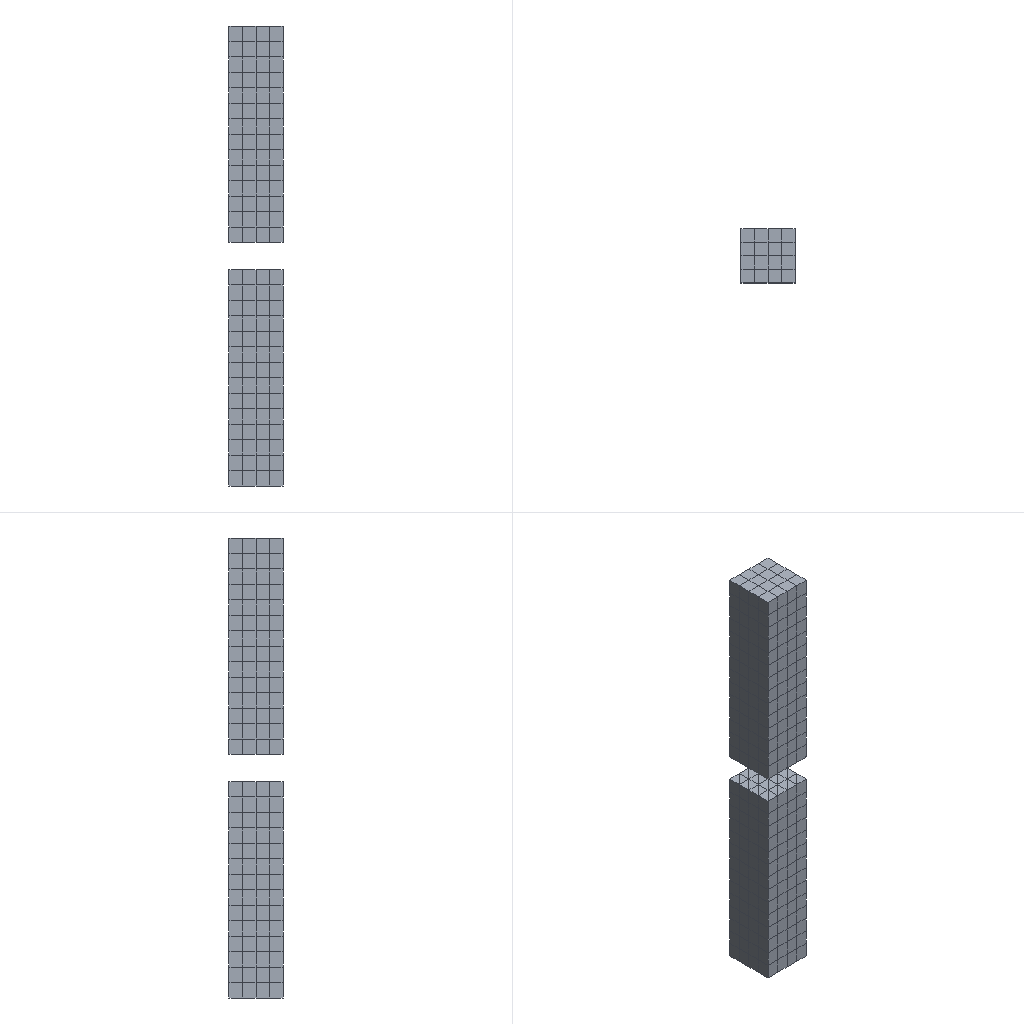Simulation study | ansys workbench
Ansys APDL input file, long lists of numbers shortened:
/batch
/config,noeldb,1     ! force off writing results to database
*get,_wallstrt,active,,time,wall
! ANSYS input file written by Workbench version 16.0 RELEASE
! File used for geometry attach: C:\Users\USE\AppData\Local\Temp\WB_LAPTOP-92PEKBNI_hmm_2756_2\unsaved_project_files\dp0\SYS\DM\SYS.agdb
/title,unsaved_project--Transient (B5)
*DIM,_wb_ProjectScratch_dir,string,248
_wb_ProjectScratch_dir(1) = 'C:\Users\USE\AppData\Local\Temp\WB_LAPTOP-92PEKBNI_hmm_2756_2\_ProjectScratch\Scr97FA\'
*DIM,_wb_SolverFiles_dir,string,248
_wb_SolverFiles_dir(1) = 'C:\Users\USE\AppData\Local\Temp\WB_LAPTOP-92PEKBNI_hmm_2756_2\unsaved_project_files\dp0\SYS-1\MECH\'
*DIM,_wb_userfiles_dir,string,248
_wb_userfiles_dir(1) = 'C:\Users\USE\AppData\Local\Temp\WB_LAPTOP-92PEKBNI_hmm_2756_2\unsaved_project_files\user_files\'
/com,--- Data in consistent NMM units. See Solving Units in the help system for more information.
/units,MPA
/nopr
/wb,file,start              !  signify a WB generated input file
/prep7
! Turn off shape checking because checks already performed inside WB mesher.
! See help system for more information.
SHPP,OFF,,NOWARN
/nolist
etcon,set             ! allow ANSYS to choose best KEYOP's for 180x elements
/com,*********** Nodes for the whole assembly ***********
nblock,3
(1i9,3e20.9e3)
        1   -2.500000000E+000    2.500000000E+000    2.857142857E+000
! (2649 more lines like these left out)
-1
/wb,elem,start            !  set before creation of elements
/com,*********** Elements for Body 1 "Solid" ***********
et,1,186
keyo,1,2,1          ! set full integration on SOLID186
eblock,19,solid,,224
(19i9)
        1        1        1        1        0        0        0        0       20        0        1        1      366      286      270      156      375      287      283
! (447 more lines like these left out)
-1
/com,*********** Elements for Body 2 "Solid" ***********
et,2,186
keyo,2,2,1          ! set full integration on SOLID186
eblock,19,solid,,224
(19i9)
        2        2        2        2        0        0        0        0       20        0      225     1326     1679     1615     1557     1481     1688     1616     1596
! (447 more lines like these left out)
-1
/wb,elem,end               !  done creating elements
/com,*********** Send User Defined Coordinate System(s) ***********
csys,0
toffst,273.15,  ! Temperature offset from absolute zero
/com,*********** Set Reference Temperature ***********
tref,22.
/wb,mat,start              !  starting to send materials
/com,*********** Send Materials ***********
MP,DENS,1,7.85e-09,	! tonne mm^-3
MP,ALPX,1,1.2e-05,	! C^-1
MP,C,1,434000000,	! mm^2 s^-2 C^-1
MP,KXX,1,60.5,	! tonne mm s^-3 C^-1
MP,RSVX,1,0.00017,	! ohm mm
MP,EX,1,200000,	! tonne s^-2 mm^-1
MP,NUXY,1,0.3,
MP,MURX,1,10000,
MP,DENS,2,7.85e-09,	! tonne mm^-3
MP,ALPX,2,1.2e-05,	! C^-1
MP,C,2,434000000,	! mm^2 s^-2 C^-1
MP,KXX,2,60.5,	! tonne mm s^-3 C^-1
MP,RSVX,2,0.00017,	! ohm mm
MP,EX,2,200000,	! tonne s^-2 mm^-1
MP,NUXY,2,0.3,
MP,MURX,2,10000,
/wb,mat,end                !  done sending materials
!************************* Model Summary ********************
!Solid,	Structural Steel,	matid,	1
!Solid,	Structural Steel,	matid,	2
!************************* End Model Summary ********************
! get the diagonal of the bounding box. Needed later for other things
*get,_xmin,node,,mnloc,x
*get,_ymin,node,,mnloc,y
*get,_zmin,node,,mnloc,z
*get,_xmax,node,,mxloc,x
*get,_ymax,node,,mxloc,y
*get,_zmax,node,,mxloc,z
_ASMDIAG=(_xmax-_xmin)*(_xmax-_xmin)+(_ymax-_ymin)*(_ymax-_ymin)+(_zmax-_zmin)*(_zmax-_zmin)
_ASMDIAG=SQRT(_ASMDIAG)
/wb,contact,start          !  starting to send contact
/com,*********** Create Contact "Frictional - Solid To Solid" ***********
/com,            Real Constant Set For Above Contact Is 4 & 3
*set,tid,4
*set,cid,3
r,tid
r,cid
et,tid,170
et,cid,174
eblock,10,,,16
(15i9)
      449        4        4        4        0      345      364      373      344     1281     1311     1279     1278
! (15 more lines like these left out)
-1
eblock,10,,,16
(15i9)
      465        3        3        3        0      345      364      373      344     1281     1311     1279     1278
! (15 more lines like these left out)
-1
eblock,10,,,16
(15i9)
      481        3        4        3        0     1672     1689     1521     1527     2609     2329     2328     2342
! (15 more lines like these left out)
-1
eblock,10,,,16
(15i9)
      497        4        3        4        0     1672     1689     1521     1527     2609     2329     2328     2342
! (15 more lines like these left out)
-1
keyo,cid,8,2               ! auto create asymmetric contact (from Program Controlled setting)
keyo,cid,10,2              ! adjust contact stiffness each NR iteration (from Program Controlled setting)
keyo,cid,12,0              ! standard contact
mp,mu,cid,0.1	! unitless
keyo,cid,2,0               ! augmented Lagrange (from Program Controlled setting)
keyo,cid,4,0               ! on Gauss point (from Program Controlled setting)
keyo,cid,9,1               ! ignore initial gaps/penetration
keyo,cid,5,1               ! auto CNOF adjustment to close geometric gap only
keyo,cid,7,0               ! No Prediction
rmod,tid,3,1.	! FKN
rmod,tid,5,0.	! ICONT
rmod,tid,6,0.	! PINB
rmod,tid,10,0.	! CNOF
rmod,tid,12,0.	! FKT
rmod,tid,36,32	! WB DSID
rmod,cid,3,1.	! FKN
rmod,cid,5,0.	! ICONT
rmod,cid,6,0.	! PINB
rmod,cid,10,0.	! CNOF
rmod,cid,12,0.	! FKT
rmod,cid,36,32	! WB DSID
nsel,all
esel,all
/wb,contact,end            !  done creating contacts
/golist
/wb,load,start             !  starting to send loads
/com,*********** Fixed Supports ***********
CMBLOCK,_FIXEDSU,NODE,       65
(8i10)
       199       200       201       216       231       288       289       290
! (8 more lines like these left out)
cmsel,s,_FIXEDSU
d,all,all
nsel,all
/com,******* Constant Zero Displacement X *******
CMBLOCK,_DISPZEROUX,NODE,       65
(8i10)
      1521      1522      1523      1527      1542      1609      1610      1611
! (8 more lines like these left out)
cmsel,s,_DISPZEROUX
d,all,ux,0
nsel,all
/com,******* Constant Zero Displacement Y *******
CMBLOCK,_DISPZEROUY,NODE,       65
(8i10)
      1521      1522      1523      1527      1542      1609      1610      1611
! (8 more lines like these left out)
cmsel,s,_DISPZEROUY
d,all,uy,0
nsel,all
nsel,all
/com,*********** Create Displacement Tables and Functions ******
*DIM,_loadvari37xp,TABLE,1,1,1,TIME,
! Time values
_loadvari37xp(1,0,1) = 1.
! Load values
_loadvari37xp(1,1,1) = 0.
*DIM,_loadvari37xn,TABLE,1,1,1,TIME,
! Time values
_loadvari37xn(1,0,1) = 1.
! Load values
_loadvari37xn(1,1,1) = -0.
*DIM,_loadvari37yp,TABLE,1,1,1,TIME,
! Time values
_loadvari37yp(1,0,1) = 1.
! Load values
_loadvari37yp(1,1,1) = 0.
*DIM,_loadvari37yn,TABLE,1,1,1,TIME,
! Time values
_loadvari37yn(1,0,1) = 1.
! Load values
_loadvari37yn(1,1,1) = -0.
*DIM,_loadvari37zp,TABLE,2,1,1,TIME,
! Time values
_loadvari37zp(1,0,1) = 0.
_loadvari37zp(2,0,1) = 1.
! Load values
_loadvari37zp(1,1,1) = 0.
_loadvari37zp(2,1,1) = 6.
*DIM,_loadvari37zn,TABLE,2,1,1,TIME,
! Time values
_loadvari37zn(1,0,1) = 0.
_loadvari37zn(2,0,1) = 1.
! Load values
_loadvari37zn(1,1,1) = -0.
_loadvari37zn(2,1,1) = -6.
/gst,on,on
fini
*get,_numnode,node,0,count
*get,_numelem,elem,0,count
*get, _MAXELEMNUM, elem, 0, NUM, MAX
*get, _MAXNODENUM, node, 0, NUM, MAX
*get, _MAXELEMTYPE, etyp, 0, NUM, MAX
*get, _MAXREALCONST, real, 0, NUM, MAX
/go
/wb,load,end               !  done creating loads
/com,--- Number of total nodes = %_numnode%
/com,--- Number of contact elements = 64
/com,--- Number of spring elements = 0
/com,--- Number of bearing elements = 0
/com,--- Number of solid elements = 448
/com,--- Number of total elements = %_numelem%
*get,_wallbsol,active,,time,wall
/com,****************************************************************************
/com,*************************    SOLUTION       ********************************
/com,****************************************************************************
/solu
antype,4                   ! transient analysis
nlgeom,on                  ! Turn on Large Deformation Effects
kbc,1                      ! stepped BC's
eqsl,pcg,1e-8,,,,,,1
cntr,print,1               ! print out contact info and also make no initial contact an error
trnopt,full,,,,,hht        ! HHT time integration method
tintp,0.1	! Numerical Damping
nldiag,cont,iter           ! print out contact info each equilibrium iteration
resc,define,last,last,,dele	   ! Program Controlled
/com,****************************************************
/com,******************* SOLVE FOR LS 1 ****************
/com,*** Set Displacements ***
CMBLOCK,_CM37UZ_ZP,NODE,       65
(8i10)
      1521      1522      1523      1527      1542      1609      1610      1611
! (8 more lines like these left out)
cmsel,s,_CM37UZ_ZP
d,all,uz,%_loadvari37zp%
nsel,all
/nopr
/gopr
autots,on                   ! User turned on automatic time stepping
deltim,0.1,0.1,0.1,OFF
time,1.
timint,on                  ! Turn on time integration effects
outres,erase
outres,all,none
outres,nsol,all
outres,rsol,all
outres,strs,all
outres,epel,all
outres,eppl,all
outres,v,all
outres,a,all
stabilize,off                   ! Stabilization turned OFF by user
! *********** WB SOLVE COMMAND ***********
! check interactive state
*get,ANSINTER_,active,,int
*if,ANSINTER_,ne,0,then
/eof
*endif
solve
/com *************** Write FE CONNECTORS *********
CEWRITE,file,ce,,INTE
/com,****************************************************
/com,*************** FINISHED SOLVE FOR LS 1 *************
*set,_DS_PROGRESS          ! turn off progress updates to avoid virus scanning bug
*get,_wallasol,active,,time,wall
/nopr
*get,_numnode,node,0,count
*get,_numelem,elem,0,count
*get, _MAXELEMNUM, elem, 0, NUM, MAX
*get, _MAXNODENUM, node, 0, NUM, MAX,,,INTERNAL
*get, _MAXELEMTYPE, etyp, 0, NUM, MAX
*get, _MAXREALCONST, real, 0, NUM, MAX
/gopr
*get,_PCGITER,active,,solu,cgiter
/post1
xmlo,ENCODING,ISO-8859-1
xmlo,parm
/xml,parm,xml
fini
/gopr
*get,_walldone,active,,time,wall
_preptime=(_wallbsol-_wallstrt)*3600
_solvtime=(_wallasol-_wallbsol)*3600
_posttime=(_walldone-_wallasol)*3600
_totaltim=(_walldone-_wallstrt)*3600
/wb,file,end               ! done with WB generated input